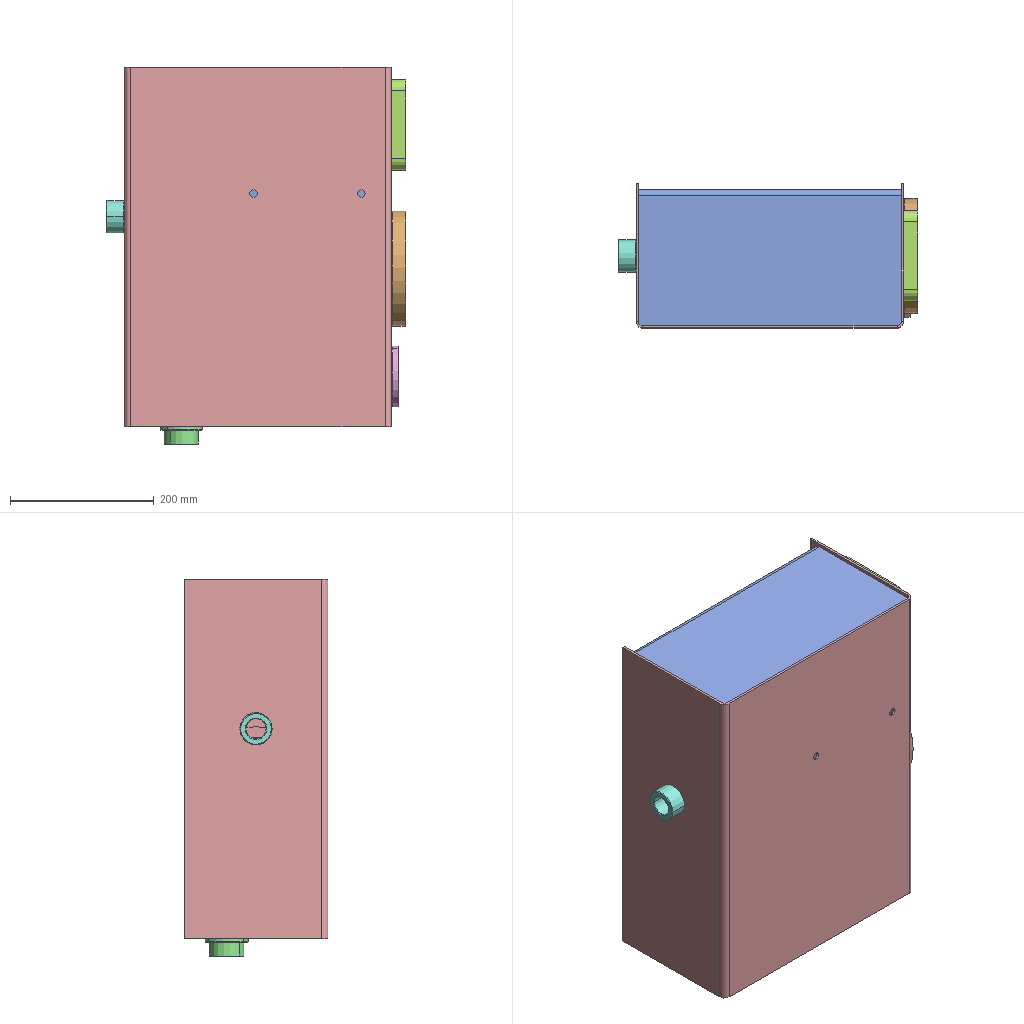Assembly | SolidWorks | 8 different items | 8 placed | box 417 x 200 x 525 mm
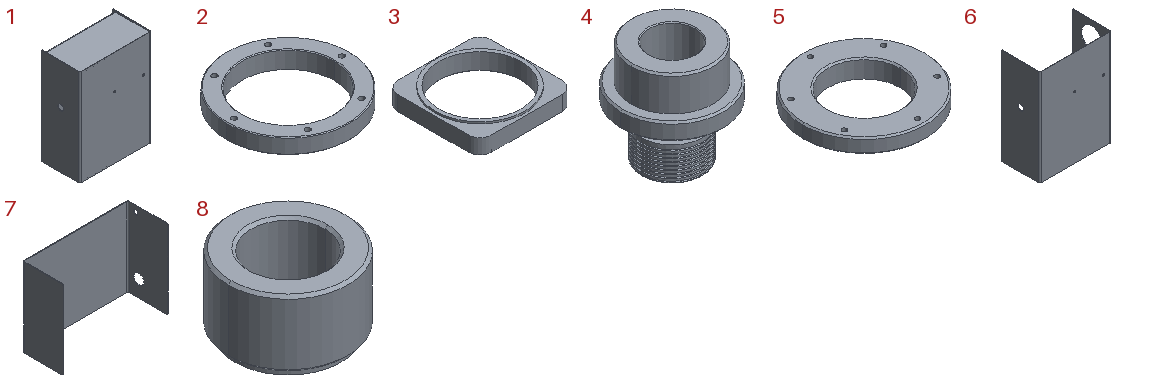Parts list (item | name | quantity | parent item | size | volume | features):
1 | (subassembly) | x1 | - | 372 x 200 x 500 mm | 2001203 mm3 | -
2 | - | x1 | - | 160 x 160 x 22.5 mm | 187073 mm3 | features 3DProfileFeature 1, Chamfer 1, Extrusion 1, HoleWzd 1, ICE 1
3 | - | x1 | - | 126 x 126 x 22.5 mm | 124484 mm3 | features 3DProfileFeature 1, Chamfer 1, Extrusion 1, HoleWzd 1, ICE 1
4 | - | x1 | - | 60 x 60 x 60 mm | 59029 mm3 | -
5 | - | x1 | - | 85 x 85 x 12.5 mm | 41153 mm3 | features 3DProfileFeature 1, Chamfer 1, Extrusion 1, HoleWzd 1, ICE 1
6 | - | x1 | in 1 | 372 x 200 x 500 mm | 1068373 mm3 | features Cut 4, FlatPattern 1, SMBaseFlange 1, SheetMetal 1
7 | - | x1 | in 1 | 490 x 189 x 366 mm | 932829 mm3 | features ICE 3, Cut 1, FlatPattern 1, SMBaseFlange 1, SheetMetal 1
8 | - | x1 | - | 45 x 45 x 27.5 mm | 25785 mm3 | features 3DProfileFeature 1, Chamfer 1, Extrusion 1, HoleWzd 1, ICE 1
Mates (type | each side: item.copy, entity, surface, feature):
In the top assembly
Parallel | 6.1 face plane Base-Flange1 | 3.1 face plane Boss-Extrude1
Coincident | 6.1 face plane Base-Flange1 | 2.1 face plane Boss-Extrude1
Coincident | 6.1 face plane Base-Flange1 | 5.1 face plane Boss-Extrude1
Coincident | 6.1 face plane Base-Flange1 | 3.1 face plane Boss-Extrude1
Coincident | 7.1 face plane Base-Flange1 | 4.1 face plane Boss-Extrude2
Coincident | 6.1 face plane Base-Flange1 | 8.1 face plane Boss-Extrude2
Concentric | 6.1 edge | 2.1 edge
Concentric | 6.1 edge | 5.1 edge
Concentric | 6.1 edge | 3.1 edge
Concentric | 6.1 edge | 8.1 select_type:24
In subassembly 1
DistanceDim | 7.2 face plane Base-Flange1 | 6.2 face plane Base-Flange1
Coincident | 6.2 face plane Base-Flange1 | 7.2 face plane Cut-Extrude2
Coincident | 6.2 face plane Base-Flange1 | 7.2 face plane Base-Flange1